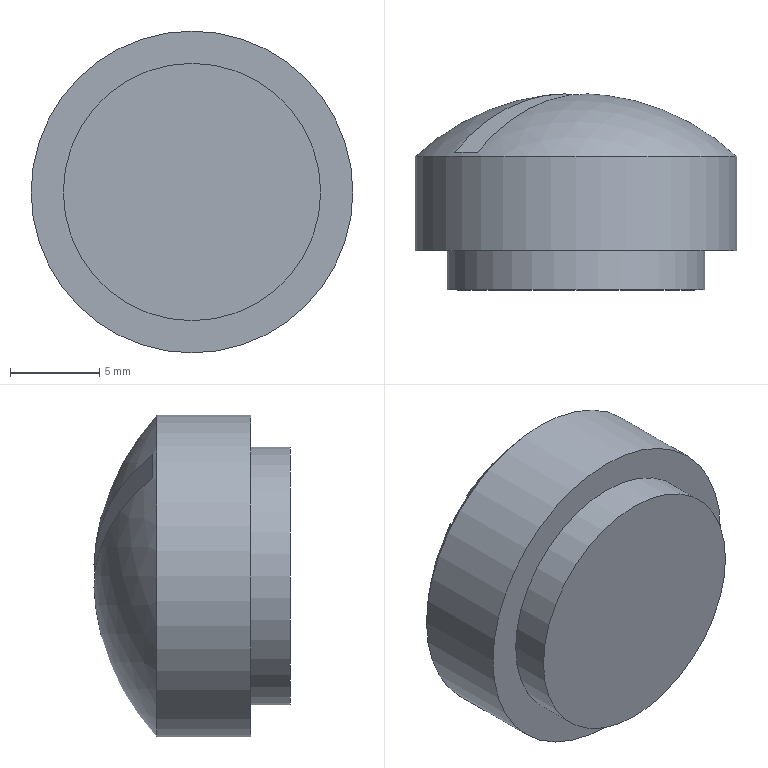Part | STEP file | basic_gh_motor_gh1_12 | 1 solid | 8 faces | box 18 x 10.969 x 18 mm | volume 2099 mm3 | plane 5 | cylinder 2 | sphere 1 | commonest cylinder face diameters 14.4 x1 18 x1
STEP:
#1=CARTESIAN_POINT('',(-69.923,139.3,-5.504));
#2=VERTEX_POINT('',#1);
#3=CARTESIAN_POINT('',(-82.204,139.3,6.777));
#4=VERTEX_POINT('',#3);
#5=CARTESIAN_POINT('',(-76.064,129.4,0.6364));
#6=DIRECTION('',(0.7071,0.,0.7071));
#7=DIRECTION('',(0.,1.,0.));
#8=AXIS2_PLACEMENT_3D('',#5,#6,#7);
#9=CIRCLE('',#8,13.169);
#10=EDGE_CURVE('',#2,#4,#9,.T.);
#11=ORIENTED_EDGE('',*,*,#10,.F.);
#12=CARTESIAN_POINT('',(-76.064,139.3,0.6364));
#13=DIRECTION('',(0.7071,0.,-0.7071));
#14=VECTOR('',#13,1.);
#15=LINE('',#12,#14);
#16=EDGE_CURVE('',#4,#2,#15,.T.);
#17=ORIENTED_EDGE('',*,*,#16,.F.);
#18=EDGE_LOOP('',(#11,#17));
#19=FACE_OUTER_BOUND('',#18,.T.);
#20=CARTESIAN_POINT('',(-76.064,144.8,0.6364));
#21=DIRECTION('',(0.7071,0.,0.7071));
#22=DIRECTION('',(0.7071,0.,-0.7071));
#23=AXIS2_PLACEMENT_3D('',#20,#21,#22);
#24=PLANE('',#23);
#25=ADVANCED_FACE('',(#19),#24,.F.);
#26=CARTESIAN_POINT('',(-83.477,139.3,5.504));
#27=VERTEX_POINT('',#26);
#28=CARTESIAN_POINT('',(-71.196,139.3,-6.777));
#29=VERTEX_POINT('',#28);
#30=CARTESIAN_POINT('',(-77.336,129.4,-0.6364));
#31=DIRECTION('',(-0.7071,0.,-0.7071));
#32=DIRECTION('',(0.,-1.,0.));
#33=AXIS2_PLACEMENT_3D('',#30,#31,#32);
#34=CIRCLE('',#33,13.169);
#35=EDGE_CURVE('',#27,#29,#34,.T.);
#36=ORIENTED_EDGE('',*,*,#35,.F.);
#37=CARTESIAN_POINT('',(-77.336,139.3,-0.6364));
#38=DIRECTION('',(-0.7071,0.,0.7071));
#39=VECTOR('',#38,1.);
#40=LINE('',#37,#39);
#41=EDGE_CURVE('',#29,#27,#40,.T.);
#42=ORIENTED_EDGE('',*,*,#41,.F.);
#43=EDGE_LOOP('',(#36,#42));
#44=FACE_OUTER_BOUND('',#43,.T.);
#45=CARTESIAN_POINT('',(-77.336,144.8,-0.6364));
#46=DIRECTION('',(0.7071,0.,0.7071));
#47=DIRECTION('',(0.7071,0.,-0.7071));
#48=AXIS2_PLACEMENT_3D('',#45,#46,#47);
#49=PLANE('',#48);
#50=ADVANCED_FACE('',(#44),#49,.T.);
#51=CARTESIAN_POINT('',(-76.7,139.3,0.));
#52=DIRECTION('',(0.,-1.,0.));
#53=DIRECTION('',(0.,0.,1.));
#54=AXIS2_PLACEMENT_3D('',#51,#52,#53);
#55=CIRCLE('',#54,8.731);
#56=EDGE_CURVE('',#29,#2,#55,.T.);
#57=ORIENTED_EDGE('',*,*,#56,.F.);
#58=ORIENTED_EDGE('',*,*,#41,.T.);
#59=CARTESIAN_POINT('',(-76.7,139.3,0.));
#60=DIRECTION('',(0.,-1.,0.));
#61=DIRECTION('',(0.,0.,1.));
#62=AXIS2_PLACEMENT_3D('',#59,#60,#61);
#63=CIRCLE('',#62,8.731);
#64=EDGE_CURVE('',#4,#27,#63,.T.);
#65=ORIENTED_EDGE('',*,*,#64,.F.);
#66=ORIENTED_EDGE('',*,*,#16,.T.);
#67=EDGE_LOOP('',(#57,#58,#65,#66));
#68=FACE_OUTER_BOUND('',#67,.T.);
#69=CARTESIAN_POINT('',(-76.7,139.3,0.));
#70=DIRECTION('',(0.,1.,0.));
#71=DIRECTION('',(0.7071,0.,0.7071));
#72=AXIS2_PLACEMENT_3D('',#69,#70,#71);
#73=PLANE('',#72);
#74=ADVANCED_FACE('',(#68),#73,.T.);
#75=CARTESIAN_POINT('',(-83.9,133.8,0.));
#76=VERTEX_POINT('',#75);
#77=CARTESIAN_POINT('',(-76.7,133.8,0.));
#78=DIRECTION('',(0.,1.,0.));
#79=DIRECTION('',(1.,0.,0.));
#80=AXIS2_PLACEMENT_3D('',#77,#78,#79);
#81=CIRCLE('',#80,7.2);
#82=EDGE_CURVE('',#76,#76,#81,.T.);
#83=ORIENTED_EDGE('',*,*,#82,.F.);
#84=CARTESIAN_POINT('',(-83.9,131.6,0.));
#85=VERTEX_POINT('',#84);
#86=CARTESIAN_POINT('',(-83.9,132.7,0.));
#87=DIRECTION('',(0.,-1.,0.));
#88=VECTOR('',#87,7.2);
#89=LINE('',#86,#88);
#90=EDGE_CURVE('',#76,#85,#89,.T.);
#91=ORIENTED_EDGE('',*,*,#90,.T.);
#92=CARTESIAN_POINT('',(-76.7,131.6,0.));
#93=DIRECTION('',(0.,1.,0.));
#94=DIRECTION('',(1.,0.,0.));
#95=AXIS2_PLACEMENT_3D('',#92,#93,#94);
#96=CIRCLE('',#95,7.2);
#97=EDGE_CURVE('',#85,#85,#96,.T.);
#98=ORIENTED_EDGE('',*,*,#97,.T.);
#99=ORIENTED_EDGE('',*,*,#90,.F.);
#100=EDGE_LOOP('',(#83,#91,#98,#99));
#101=FACE_OUTER_BOUND('',#100,.T.);
#102=CARTESIAN_POINT('',(-76.7,132.7,0.));
#103=DIRECTION('',(0.,1.,0.));
#104=DIRECTION('',(1.,0.,0.));
#105=AXIS2_PLACEMENT_3D('',#102,#103,#104);
#106=CYLINDRICAL_SURFACE('',#105,7.2);
#107=ADVANCED_FACE('',(#101),#106,.T.);
#108=CARTESIAN_POINT('',(-85.7,133.8,0.));
#109=VERTEX_POINT('',#108);
#110=CARTESIAN_POINT('',(-76.7,133.8,0.));
#111=DIRECTION('',(0.,1.,0.));
#112=DIRECTION('',(1.,0.,0.));
#113=AXIS2_PLACEMENT_3D('',#110,#111,#112);
#114=CIRCLE('',#113,9.);
#115=EDGE_CURVE('',#109,#109,#114,.T.);
#116=ORIENTED_EDGE('',*,*,#115,.F.);
#117=EDGE_LOOP('',(#116));
#118=FACE_OUTER_BOUND('',#117,.T.);
#119=ORIENTED_EDGE('',*,*,#82,.T.);
#120=EDGE_LOOP('',(#119));
#121=FACE_BOUND('',#120,.T.);
#122=CARTESIAN_POINT('',(-68.6,133.8,0.));
#123=DIRECTION('',(0.,-1.,0.));
#124=DIRECTION('',(-1.,0.,0.));
#125=AXIS2_PLACEMENT_3D('',#122,#123,#124);
#126=PLANE('',#125);
#127=ADVANCED_FACE('',(#118,#121),#126,.T.);
#128=CARTESIAN_POINT('',(-85.7,139.056,0.));
#129=VERTEX_POINT('',#128);
#130=CARTESIAN_POINT('',(-76.7,139.056,0.));
#131=DIRECTION('',(0.,1.,0.));
#132=DIRECTION('',(1.,0.,0.));
#133=AXIS2_PLACEMENT_3D('',#130,#131,#132);
#134=CIRCLE('',#133,9.);
#135=EDGE_CURVE('',#129,#129,#134,.T.);
#136=ORIENTED_EDGE('',*,*,#135,.F.);
#137=CARTESIAN_POINT('',(-85.7,136.428,0.));
#138=DIRECTION('',(0.,-1.,0.));
#139=VECTOR('',#138,9.);
#140=LINE('',#137,#139);
#141=EDGE_CURVE('',#129,#109,#140,.T.);
#142=ORIENTED_EDGE('',*,*,#141,.T.);
#143=ORIENTED_EDGE('',*,*,#115,.T.);
#144=ORIENTED_EDGE('',*,*,#141,.F.);
#145=EDGE_LOOP('',(#136,#142,#143,#144));
#146=FACE_OUTER_BOUND('',#145,.T.);
#147=CARTESIAN_POINT('',(-76.7,136.428,0.));
#148=DIRECTION('',(0.,1.,0.));
#149=DIRECTION('',(1.,0.,0.));
#150=AXIS2_PLACEMENT_3D('',#147,#148,#149);
#151=CYLINDRICAL_SURFACE('',#150,9.);
#152=ADVANCED_FACE('',(#146),#151,.T.);
#153=ORIENTED_EDGE('',*,*,#135,.T.);
#154=EDGE_LOOP('',(#153));
#155=FACE_OUTER_BOUND('',#154,.T.);
#156=ORIENTED_EDGE('',*,*,#35,.T.);
#157=ORIENTED_EDGE('',*,*,#56,.T.);
#158=ORIENTED_EDGE('',*,*,#10,.T.);
#159=ORIENTED_EDGE('',*,*,#64,.T.);
#160=EDGE_LOOP('',(#156,#157,#158,#159));
#161=FACE_BOUND('',#160,.T.);
#162=CARTESIAN_POINT('',(-76.7,129.4,0.));
#163=DIRECTION('',(0.,0.,1.));
#164=DIRECTION('',(1.,0.,0.));
#165=AXIS2_PLACEMENT_3D('',#162,#163,#164);
#166=SPHERICAL_SURFACE('',#165,13.2);
#167=ADVANCED_FACE('',(#155,#161),#166,.T.);
#168=ORIENTED_EDGE('',*,*,#97,.F.);
#169=EDGE_LOOP('',(#168));
#170=FACE_OUTER_BOUND('',#169,.T.);
#171=CARTESIAN_POINT('',(-73.1,131.6,0.));
#172=DIRECTION('',(0.,-1.,0.));
#173=DIRECTION('',(-1.,0.,0.));
#174=AXIS2_PLACEMENT_3D('',#171,#172,#173);
#175=PLANE('',#174);
#176=ADVANCED_FACE('',(#170),#175,.T.);
#177=CLOSED_SHELL('',(#25,#50,#74,#107,#127,#152,#167,#176));
#178=MANIFOLD_SOLID_BREP('',#177);
#179=(LENGTH_UNIT()NAMED_UNIT(*)SI_UNIT(.MILLI.,.METRE.));
#180=UNCERTAINTY_MEASURE_WITH_UNIT(LENGTH_MEASURE(0.01),#179,'','');
#181=(NAMED_UNIT(*)PLANE_ANGLE_UNIT()SI_UNIT($,.RADIAN.));
#182=(NAMED_UNIT(*)SI_UNIT($,.STERADIAN.)SOLID_ANGLE_UNIT());
#183=(GEOMETRIC_REPRESENTATION_CONTEXT(3)GLOBAL_UNCERTAINTY_ASSIGNED_CONTEXT((#180))GLOBAL_UNIT_ASSIGNED_CONTEXT((#179,#181,#182))REPRESENTATION_CONTEXT('',''));
#184=ADVANCED_BREP_SHAPE_REPRESENTATION('',(#178),#183);